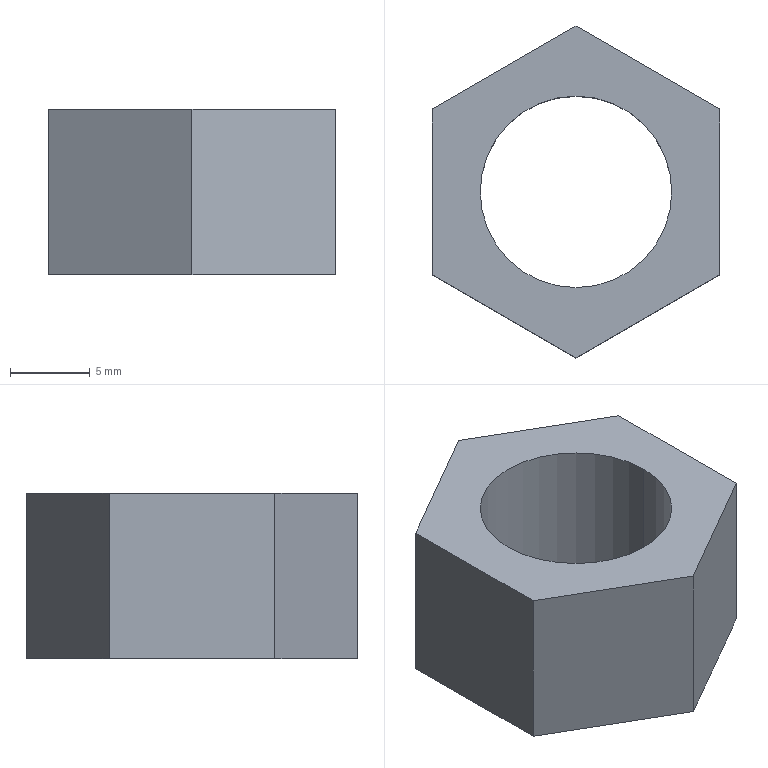Part | SolidWorks | features Extrusion 1 | 1 solid | 10 faces | box 18 x 20.785 x 10.4 mm | volume 1742 mm3 | plane 8 | cylinder 2 | commonest cylinder face diameters 12 x2
STEP:
#1=CARTESIAN_POINT('',(-6.,0.,10.4));
#2=VERTEX_POINT('',#1);
#3=CARTESIAN_POINT('',(6.,0.,10.4));
#4=VERTEX_POINT('',#3);
#5=CARTESIAN_POINT('',(0.,0.,10.4));
#6=DIRECTION('',(0.,0.,1.));
#7=DIRECTION('',(1.,0.,0.));
#8=AXIS2_PLACEMENT_3D('',#5,#6,#7);
#9=CIRCLE('',#8,6.);
#10=EDGE_CURVE('',#2,#4,#9,.T.);
#11=ORIENTED_EDGE('',*,*,#10,.T.);
#12=CARTESIAN_POINT('',(6.,0.,0.));
#13=VERTEX_POINT('',#12);
#14=CARTESIAN_POINT('',(6.,0.,10.4));
#15=DIRECTION('',(0.,0.,-1.));
#16=VECTOR('',#15,1000.);
#17=LINE('',#14,#16);
#18=EDGE_CURVE('',#4,#13,#17,.T.);
#19=ORIENTED_EDGE('',*,*,#18,.T.);
#20=CARTESIAN_POINT('',(-6.,0.,0.));
#21=VERTEX_POINT('',#20);
#22=CARTESIAN_POINT('',(0.,0.,0.));
#23=DIRECTION('',(0.,0.,1.));
#24=DIRECTION('',(1.,0.,0.));
#25=AXIS2_PLACEMENT_3D('',#22,#23,#24);
#26=CIRCLE('',#25,6.);
#27=EDGE_CURVE('',#21,#13,#26,.T.);
#28=ORIENTED_EDGE('',*,*,#27,.F.);
#29=CARTESIAN_POINT('',(-6.,0.,10.4));
#30=DIRECTION('',(0.,0.,-1.));
#31=VECTOR('',#30,1000.);
#32=LINE('',#29,#31);
#33=EDGE_CURVE('',#2,#21,#32,.T.);
#34=ORIENTED_EDGE('',*,*,#33,.F.);
#35=EDGE_LOOP('',(#11,#19,#28,#34));
#36=FACE_OUTER_BOUND('',#35,.T.);
#37=CARTESIAN_POINT('',(0.,0.,10.4));
#38=DIRECTION('',(0.,0.,-1.));
#39=DIRECTION('',(-1.,0.,0.));
#40=AXIS2_PLACEMENT_3D('',#37,#38,#39);
#41=CYLINDRICAL_SURFACE('',#40,6.);
#42=ADVANCED_FACE('',(#36),#41,.F.);
#43=CARTESIAN_POINT('',(-9.,-5.196,10.4));
#44=VERTEX_POINT('',#43);
#45=CARTESIAN_POINT('',(0.,-10.392,10.4));
#46=VERTEX_POINT('',#45);
#47=CARTESIAN_POINT('',(-9.,-5.196,10.4));
#48=DIRECTION('',(0.866,-0.5,0.));
#49=VECTOR('',#48,1000.);
#50=LINE('',#47,#49);
#51=EDGE_CURVE('',#44,#46,#50,.T.);
#52=ORIENTED_EDGE('',*,*,#51,.T.);
#53=CARTESIAN_POINT('',(9.,-5.196,10.4));
#54=VERTEX_POINT('',#53);
#55=CARTESIAN_POINT('',(0.,-10.392,10.4));
#56=DIRECTION('',(0.866,0.5,0.));
#57=VECTOR('',#56,1000.);
#58=LINE('',#55,#57);
#59=EDGE_CURVE('',#46,#54,#58,.T.);
#60=ORIENTED_EDGE('',*,*,#59,.T.);
#61=CARTESIAN_POINT('',(9.,5.196,10.4));
#62=VERTEX_POINT('',#61);
#63=CARTESIAN_POINT('',(9.,-5.196,10.4));
#64=DIRECTION('',(0.,1.,0.));
#65=VECTOR('',#64,1000.);
#66=LINE('',#63,#65);
#67=EDGE_CURVE('',#54,#62,#66,.T.);
#68=ORIENTED_EDGE('',*,*,#67,.T.);
#69=CARTESIAN_POINT('',(0.,10.392,10.4));
#70=VERTEX_POINT('',#69);
#71=CARTESIAN_POINT('',(9.,5.196,10.4));
#72=DIRECTION('',(-0.866,0.5,0.));
#73=VECTOR('',#72,1000.);
#74=LINE('',#71,#73);
#75=EDGE_CURVE('',#62,#70,#74,.T.);
#76=ORIENTED_EDGE('',*,*,#75,.T.);
#77=CARTESIAN_POINT('',(-9.,5.196,10.4));
#78=VERTEX_POINT('',#77);
#79=CARTESIAN_POINT('',(0.,10.392,10.4));
#80=DIRECTION('',(-0.866,-0.5,0.));
#81=VECTOR('',#80,1000.);
#82=LINE('',#79,#81);
#83=EDGE_CURVE('',#70,#78,#82,.T.);
#84=ORIENTED_EDGE('',*,*,#83,.T.);
#85=CARTESIAN_POINT('',(-9.,5.196,10.4));
#86=DIRECTION('',(0.,-1.,0.));
#87=VECTOR('',#86,1000.);
#88=LINE('',#85,#87);
#89=EDGE_CURVE('',#78,#44,#88,.T.);
#90=ORIENTED_EDGE('',*,*,#89,.T.);
#91=EDGE_LOOP('',(#52,#60,#68,#76,#84,#90));
#92=FACE_OUTER_BOUND('',#91,.T.);
#93=ORIENTED_EDGE('',*,*,#10,.F.);
#94=CARTESIAN_POINT('',(0.,0.,10.4));
#95=DIRECTION('',(0.,0.,1.));
#96=DIRECTION('',(1.,0.,0.));
#97=AXIS2_PLACEMENT_3D('',#94,#95,#96);
#98=CIRCLE('',#97,6.);
#99=EDGE_CURVE('',#4,#2,#98,.T.);
#100=ORIENTED_EDGE('',*,*,#99,.F.);
#101=EDGE_LOOP('',(#93,#100));
#102=FACE_BOUND('',#101,.T.);
#103=CARTESIAN_POINT('',(0.,0.,10.4));
#104=DIRECTION('',(0.,0.,1.));
#105=DIRECTION('',(1.,0.,0.));
#106=AXIS2_PLACEMENT_3D('',#103,#104,#105);
#107=PLANE('',#106);
#108=ADVANCED_FACE('',(#92,#102),#107,.T.);
#109=CARTESIAN_POINT('',(-9.,-5.196,0.));
#110=VERTEX_POINT('',#109);
#111=CARTESIAN_POINT('',(0.,-10.392,0.));
#112=VERTEX_POINT('',#111);
#113=CARTESIAN_POINT('',(-9.,-5.196,0.));
#114=DIRECTION('',(0.866,-0.5,0.));
#115=VECTOR('',#114,1000.);
#116=LINE('',#113,#115);
#117=EDGE_CURVE('',#110,#112,#116,.T.);
#118=ORIENTED_EDGE('',*,*,#117,.F.);
#119=CARTESIAN_POINT('',(-9.,5.196,0.));
#120=VERTEX_POINT('',#119);
#121=CARTESIAN_POINT('',(-9.,5.196,0.));
#122=DIRECTION('',(0.,-1.,0.));
#123=VECTOR('',#122,1000.);
#124=LINE('',#121,#123);
#125=EDGE_CURVE('',#120,#110,#124,.T.);
#126=ORIENTED_EDGE('',*,*,#125,.F.);
#127=CARTESIAN_POINT('',(0.,10.392,0.));
#128=VERTEX_POINT('',#127);
#129=CARTESIAN_POINT('',(0.,10.392,0.));
#130=DIRECTION('',(-0.866,-0.5,0.));
#131=VECTOR('',#130,1000.);
#132=LINE('',#129,#131);
#133=EDGE_CURVE('',#128,#120,#132,.T.);
#134=ORIENTED_EDGE('',*,*,#133,.F.);
#135=CARTESIAN_POINT('',(9.,5.196,0.));
#136=VERTEX_POINT('',#135);
#137=CARTESIAN_POINT('',(9.,5.196,0.));
#138=DIRECTION('',(-0.866,0.5,0.));
#139=VECTOR('',#138,1000.);
#140=LINE('',#137,#139);
#141=EDGE_CURVE('',#136,#128,#140,.T.);
#142=ORIENTED_EDGE('',*,*,#141,.F.);
#143=CARTESIAN_POINT('',(9.,-5.196,0.));
#144=VERTEX_POINT('',#143);
#145=CARTESIAN_POINT('',(9.,-5.196,0.));
#146=DIRECTION('',(0.,1.,0.));
#147=VECTOR('',#146,1000.);
#148=LINE('',#145,#147);
#149=EDGE_CURVE('',#144,#136,#148,.T.);
#150=ORIENTED_EDGE('',*,*,#149,.F.);
#151=CARTESIAN_POINT('',(0.,-10.392,0.));
#152=DIRECTION('',(0.866,0.5,0.));
#153=VECTOR('',#152,1000.);
#154=LINE('',#151,#153);
#155=EDGE_CURVE('',#112,#144,#154,.T.);
#156=ORIENTED_EDGE('',*,*,#155,.F.);
#157=EDGE_LOOP('',(#118,#126,#134,#142,#150,#156));
#158=FACE_OUTER_BOUND('',#157,.T.);
#159=ORIENTED_EDGE('',*,*,#27,.T.);
#160=CARTESIAN_POINT('',(0.,0.,0.));
#161=DIRECTION('',(0.,0.,1.));
#162=DIRECTION('',(1.,0.,0.));
#163=AXIS2_PLACEMENT_3D('',#160,#161,#162);
#164=CIRCLE('',#163,6.);
#165=EDGE_CURVE('',#13,#21,#164,.T.);
#166=ORIENTED_EDGE('',*,*,#165,.T.);
#167=EDGE_LOOP('',(#159,#166));
#168=FACE_BOUND('',#167,.T.);
#169=CARTESIAN_POINT('',(0.,0.,0.));
#170=DIRECTION('',(0.,0.,1.));
#171=DIRECTION('',(1.,0.,0.));
#172=AXIS2_PLACEMENT_3D('',#169,#170,#171);
#173=PLANE('',#172);
#174=ADVANCED_FACE('',(#158,#168),#173,.F.);
#175=ORIENTED_EDGE('',*,*,#117,.T.);
#176=CARTESIAN_POINT('',(0.,-10.392,10.4));
#177=DIRECTION('',(0.,0.,-1.));
#178=VECTOR('',#177,1000.);
#179=LINE('',#176,#178);
#180=EDGE_CURVE('',#46,#112,#179,.T.);
#181=ORIENTED_EDGE('',*,*,#180,.F.);
#182=ORIENTED_EDGE('',*,*,#51,.F.);
#183=CARTESIAN_POINT('',(-9.,-5.196,10.4));
#184=DIRECTION('',(0.,0.,-1.));
#185=VECTOR('',#184,1000.);
#186=LINE('',#183,#185);
#187=EDGE_CURVE('',#44,#110,#186,.T.);
#188=ORIENTED_EDGE('',*,*,#187,.T.);
#189=EDGE_LOOP('',(#175,#181,#182,#188));
#190=FACE_OUTER_BOUND('',#189,.T.);
#191=CARTESIAN_POINT('',(-9.,-5.196,10.4));
#192=DIRECTION('',(0.5,0.866,0.));
#193=DIRECTION('',(-0.866,0.5,0.));
#194=AXIS2_PLACEMENT_3D('',#191,#192,#193);
#195=PLANE('',#194);
#196=ADVANCED_FACE('',(#190),#195,.F.);
#197=ORIENTED_EDGE('',*,*,#155,.T.);
#198=CARTESIAN_POINT('',(9.,-5.196,10.4));
#199=DIRECTION('',(0.,0.,-1.));
#200=VECTOR('',#199,1000.);
#201=LINE('',#198,#200);
#202=EDGE_CURVE('',#54,#144,#201,.T.);
#203=ORIENTED_EDGE('',*,*,#202,.F.);
#204=ORIENTED_EDGE('',*,*,#59,.F.);
#205=ORIENTED_EDGE('',*,*,#180,.T.);
#206=EDGE_LOOP('',(#197,#203,#204,#205));
#207=FACE_OUTER_BOUND('',#206,.T.);
#208=CARTESIAN_POINT('',(0.,-10.392,10.4));
#209=DIRECTION('',(-0.5,0.866,0.));
#210=DIRECTION('',(-0.866,-0.5,0.));
#211=AXIS2_PLACEMENT_3D('',#208,#209,#210);
#212=PLANE('',#211);
#213=ADVANCED_FACE('',(#207),#212,.F.);
#214=ORIENTED_EDGE('',*,*,#149,.T.);
#215=CARTESIAN_POINT('',(9.,5.196,10.4));
#216=DIRECTION('',(0.,0.,-1.));
#217=VECTOR('',#216,1000.);
#218=LINE('',#215,#217);
#219=EDGE_CURVE('',#62,#136,#218,.T.);
#220=ORIENTED_EDGE('',*,*,#219,.F.);
#221=ORIENTED_EDGE('',*,*,#67,.F.);
#222=ORIENTED_EDGE('',*,*,#202,.T.);
#223=EDGE_LOOP('',(#214,#220,#221,#222));
#224=FACE_OUTER_BOUND('',#223,.T.);
#225=CARTESIAN_POINT('',(9.,-5.196,10.4));
#226=DIRECTION('',(-1.,0.,0.));
#227=DIRECTION('',(0.,0.,1.));
#228=AXIS2_PLACEMENT_3D('',#225,#226,#227);
#229=PLANE('',#228);
#230=ADVANCED_FACE('',(#224),#229,.F.);
#231=ORIENTED_EDGE('',*,*,#141,.T.);
#232=CARTESIAN_POINT('',(0.,10.392,10.4));
#233=DIRECTION('',(0.,0.,-1.));
#234=VECTOR('',#233,1000.);
#235=LINE('',#232,#234);
#236=EDGE_CURVE('',#70,#128,#235,.T.);
#237=ORIENTED_EDGE('',*,*,#236,.F.);
#238=ORIENTED_EDGE('',*,*,#75,.F.);
#239=ORIENTED_EDGE('',*,*,#219,.T.);
#240=EDGE_LOOP('',(#231,#237,#238,#239));
#241=FACE_OUTER_BOUND('',#240,.T.);
#242=CARTESIAN_POINT('',(9.,5.196,10.4));
#243=DIRECTION('',(-0.5,-0.866,0.));
#244=DIRECTION('',(0.866,-0.5,0.));
#245=AXIS2_PLACEMENT_3D('',#242,#243,#244);
#246=PLANE('',#245);
#247=ADVANCED_FACE('',(#241),#246,.F.);
#248=ORIENTED_EDGE('',*,*,#133,.T.);
#249=CARTESIAN_POINT('',(-9.,5.196,10.4));
#250=DIRECTION('',(0.,0.,-1.));
#251=VECTOR('',#250,1000.);
#252=LINE('',#249,#251);
#253=EDGE_CURVE('',#78,#120,#252,.T.);
#254=ORIENTED_EDGE('',*,*,#253,.F.);
#255=ORIENTED_EDGE('',*,*,#83,.F.);
#256=ORIENTED_EDGE('',*,*,#236,.T.);
#257=EDGE_LOOP('',(#248,#254,#255,#256));
#258=FACE_OUTER_BOUND('',#257,.T.);
#259=CARTESIAN_POINT('',(0.,10.392,10.4));
#260=DIRECTION('',(0.5,-0.866,0.));
#261=DIRECTION('',(0.866,0.5,0.));
#262=AXIS2_PLACEMENT_3D('',#259,#260,#261);
#263=PLANE('',#262);
#264=ADVANCED_FACE('',(#258),#263,.F.);
#265=ORIENTED_EDGE('',*,*,#125,.T.);
#266=ORIENTED_EDGE('',*,*,#187,.F.);
#267=ORIENTED_EDGE('',*,*,#89,.F.);
#268=ORIENTED_EDGE('',*,*,#253,.T.);
#269=EDGE_LOOP('',(#265,#266,#267,#268));
#270=FACE_OUTER_BOUND('',#269,.T.);
#271=CARTESIAN_POINT('',(-9.,5.196,10.4));
#272=DIRECTION('',(1.,0.,0.));
#273=DIRECTION('',(0.,1.,0.));
#274=AXIS2_PLACEMENT_3D('',#271,#272,#273);
#275=PLANE('',#274);
#276=ADVANCED_FACE('',(#270),#275,.F.);
#277=ORIENTED_EDGE('',*,*,#18,.F.);
#278=ORIENTED_EDGE('',*,*,#99,.T.);
#279=ORIENTED_EDGE('',*,*,#33,.T.);
#280=ORIENTED_EDGE('',*,*,#165,.F.);
#281=EDGE_LOOP('',(#277,#278,#279,#280));
#282=FACE_OUTER_BOUND('',#281,.T.);
#283=CARTESIAN_POINT('',(0.,0.,10.4));
#284=DIRECTION('',(0.,0.,-1.));
#285=DIRECTION('',(-1.,0.,0.));
#286=AXIS2_PLACEMENT_3D('',#283,#284,#285);
#287=CYLINDRICAL_SURFACE('',#286,6.);
#288=ADVANCED_FACE('',(#282),#287,.F.);
#289=CLOSED_SHELL('',(#42,#108,#174,#196,#213,#230,#247,#264,#276,#288));
#290=MANIFOLD_SOLID_BREP('',#289);
#291=CARTESIAN_POINT('',(0.,0.,0.));
#292=DIRECTION('',(0.,0.,1.));
#293=DIRECTION('',(1.,0.,0.));
#294=AXIS2_PLACEMENT_3D('',#291,#292,#293);
#295=(LENGTH_UNIT()NAMED_UNIT(*)SI_UNIT(.MILLI.,.METRE.));
#296=UNCERTAINTY_MEASURE_WITH_UNIT(LENGTH_MEASURE(0.00001),#295,'','');
#297=(NAMED_UNIT(*)PLANE_ANGLE_UNIT()SI_UNIT($,.RADIAN.));
#298=(NAMED_UNIT(*)SI_UNIT($,.STERADIAN.)SOLID_ANGLE_UNIT());
#299=(GEOMETRIC_REPRESENTATION_CONTEXT(3)GLOBAL_UNCERTAINTY_ASSIGNED_CONTEXT((#296))GLOBAL_UNIT_ASSIGNED_CONTEXT((#295,#297,#298))REPRESENTATION_CONTEXT('',''));
#300=ADVANCED_BREP_SHAPE_REPRESENTATION('',(#290,#294),#299);